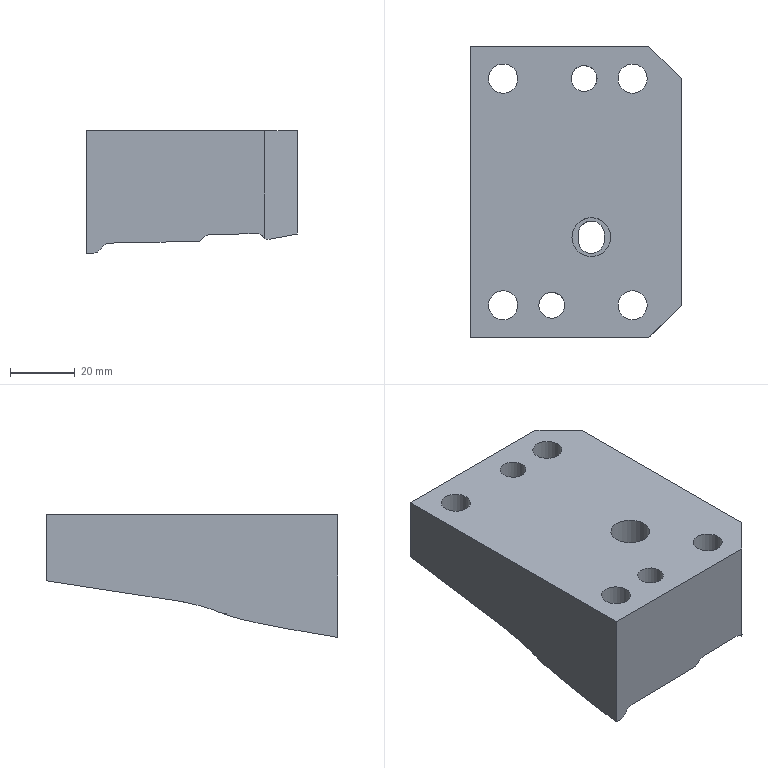Part | NX | features solid 2 | 1 solid | 54 faces | box 65 x 90 x 37.916 mm | volume 134615 mm3 | spline 27 | plane 14 | cylinder 13 | commonest cylinder face diameters 8 x4 9 x4 14 x4 12 x1